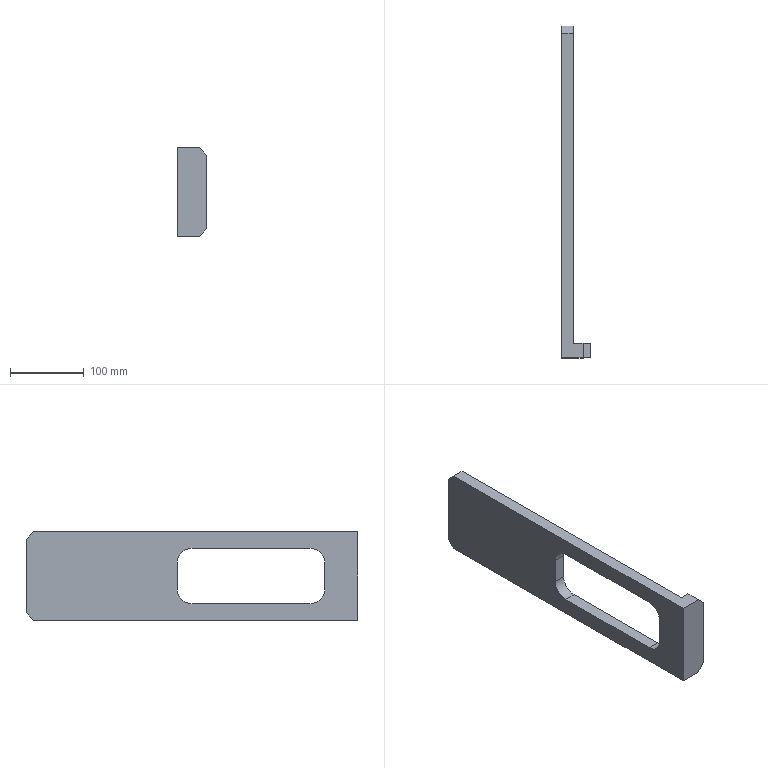Part | STEP file | PN_0019 | 1 solid | 20 faces | box 39.2 x 450 x 120 mm | volume 681574 mm3 | plane 16 | cylinder 4 | commonest cylinder face diameters 40 x4
STEP:
#1=CARTESIAN_POINT('',(0.,0.,0.));
#2=DIRECTION('',(0.,0.,1.));
#3=DIRECTION('',(1.,0.,0.));
#4=AXIS2_PLACEMENT_3D('',#1,#2,#3);
#5=CARTESIAN_POINT('',(0.,225.,97.5));
#6=VERTEX_POINT('',#5);
#7=CARTESIAN_POINT('',(0.,65.,97.5));
#8=VERTEX_POINT('',#7);
#9=CARTESIAN_POINT('',(0.,0.,97.5));
#10=DIRECTION('',(0.,-1.,0.));
#11=VECTOR('',#10,1.);
#12=LINE('',#9,#11);
#13=CARTESIAN_POINT('',(0.,0.,120.));
#14=DIRECTION('',(1.,0.,0.));
#15=DIRECTION('',(0.,0.,-1.));
#16=AXIS2_PLACEMENT_3D('',#13,#14,#15);
#17=PLANE('',#16);
#18=CARTESIAN_POINT('',(22.5,0.));
#19=DIRECTION('',(0.,-1.));
#20=VECTOR('',#19,1.);
#21=LINE('',#18,#20);
#22=(GEOMETRIC_REPRESENTATION_CONTEXT(2)PARAMETRIC_REPRESENTATION_CONTEXT()REPRESENTATION_CONTEXT('',''));
#23=DEFINITIONAL_REPRESENTATION('',(#21),#22);
#24=PCURVE('',#17,#23);
#25=CARTESIAN_POINT('',(-104.,245.,97.5));
#26=DIRECTION('',(0.,0.,1.));
#27=DIRECTION('',(0.,-1.,0.));
#28=AXIS2_PLACEMENT_3D('',#25,#26,#27);
#29=PLANE('',#28);
#30=CARTESIAN_POINT('',(245.,104.));
#31=DIRECTION('',(1.,0.));
#32=VECTOR('',#31,1.);
#33=LINE('',#30,#32);
#34=(GEOMETRIC_REPRESENTATION_CONTEXT(2)PARAMETRIC_REPRESENTATION_CONTEXT()REPRESENTATION_CONTEXT('',''));
#35=DEFINITIONAL_REPRESENTATION('',(#33),#34);
#36=PCURVE('',#29,#35);
#37=SURFACE_CURVE('',#12,(#24,#36),.PCURVE_S1.);
#38=EDGE_CURVE('',#6,#8,#37,.T.);
#39=ORIENTED_EDGE('',*,*,#38,.T.);
#40=CARTESIAN_POINT('',(0.,45.,77.5));
#41=VERTEX_POINT('',#40);
#42=CARTESIAN_POINT('',(0.,65.,77.5));
#43=DIRECTION('',(1.,0.,0.));
#44=DIRECTION('',(0.,0.,-1.));
#45=AXIS2_PLACEMENT_3D('',#42,#43,#44);
#46=CIRCLE('',#45,20.);
#47=CARTESIAN_POINT('',(42.5,65.));
#48=DIRECTION('',(1.,0.));
#49=AXIS2_PLACEMENT_2D('',#47,#48);
#50=CIRCLE('',#49,20.);
#51=(GEOMETRIC_REPRESENTATION_CONTEXT(2)PARAMETRIC_REPRESENTATION_CONTEXT()REPRESENTATION_CONTEXT('',''));
#52=DEFINITIONAL_REPRESENTATION('',(#50),#51);
#53=PCURVE('',#17,#52);
#54=CARTESIAN_POINT('',(-104.,65.,77.5));
#55=DIRECTION('',(-1.,0.,0.));
#56=DIRECTION('',(0.,-1.,0.));
#57=AXIS2_PLACEMENT_3D('',#54,#55,#56);
#58=CYLINDRICAL_SURFACE('',#57,20.);
#59=CARTESIAN_POINT('',(4.712,-104.));
#60=DIRECTION('',(-1.,0.));
#61=VECTOR('',#60,1.);
#62=LINE('',#59,#61);
#63=(GEOMETRIC_REPRESENTATION_CONTEXT(2)PARAMETRIC_REPRESENTATION_CONTEXT()REPRESENTATION_CONTEXT('',''));
#64=DEFINITIONAL_REPRESENTATION('',(#62),#63);
#65=PCURVE('',#58,#64);
#66=SURFACE_CURVE('',#46,(#53,#65),.PCURVE_S1.);
#67=EDGE_CURVE('',#8,#41,#66,.T.);
#68=ORIENTED_EDGE('',*,*,#67,.T.);
#69=CARTESIAN_POINT('',(0.,45.,42.5));
#70=VERTEX_POINT('',#69);
#71=CARTESIAN_POINT('',(0.,45.,120.));
#72=DIRECTION('',(0.,0.,-1.));
#73=VECTOR('',#72,1.);
#74=LINE('',#71,#73);
#75=CARTESIAN_POINT('',(0.,45.));
#76=DIRECTION('',(1.,0.));
#77=VECTOR('',#76,1.);
#78=LINE('',#75,#77);
#79=(GEOMETRIC_REPRESENTATION_CONTEXT(2)PARAMETRIC_REPRESENTATION_CONTEXT()REPRESENTATION_CONTEXT('',''));
#80=DEFINITIONAL_REPRESENTATION('',(#78),#79);
#81=PCURVE('',#17,#80);
#82=CARTESIAN_POINT('',(-104.,45.,97.5));
#83=DIRECTION('',(0.,-1.,0.));
#84=DIRECTION('',(0.,0.,-1.));
#85=AXIS2_PLACEMENT_3D('',#82,#83,#84);
#86=PLANE('',#85);
#87=CARTESIAN_POINT('',(-22.5,104.));
#88=DIRECTION('',(1.,0.));
#89=VECTOR('',#88,1.);
#90=LINE('',#87,#89);
#91=(GEOMETRIC_REPRESENTATION_CONTEXT(2)PARAMETRIC_REPRESENTATION_CONTEXT()REPRESENTATION_CONTEXT('',''));
#92=DEFINITIONAL_REPRESENTATION('',(#90),#91);
#93=PCURVE('',#86,#92);
#94=SURFACE_CURVE('',#74,(#81,#93),.PCURVE_S1.);
#95=EDGE_CURVE('',#41,#70,#94,.T.);
#96=ORIENTED_EDGE('',*,*,#95,.T.);
#97=CARTESIAN_POINT('',(0.,65.,22.5));
#98=VERTEX_POINT('',#97);
#99=CARTESIAN_POINT('',(0.,65.,42.5));
#100=DIRECTION('',(1.,0.,0.));
#101=DIRECTION('',(0.,0.,-1.));
#102=AXIS2_PLACEMENT_3D('',#99,#100,#101);
#103=CIRCLE('',#102,20.);
#104=CARTESIAN_POINT('',(77.5,65.));
#105=DIRECTION('',(1.,0.));
#106=AXIS2_PLACEMENT_2D('',#104,#105);
#107=CIRCLE('',#106,20.);
#108=(GEOMETRIC_REPRESENTATION_CONTEXT(2)PARAMETRIC_REPRESENTATION_CONTEXT()REPRESENTATION_CONTEXT('',''));
#109=DEFINITIONAL_REPRESENTATION('',(#107),#108);
#110=PCURVE('',#17,#109);
#111=CARTESIAN_POINT('',(-104.,65.,42.5));
#112=DIRECTION('',(-1.,0.,0.));
#113=DIRECTION('',(0.,-1.,0.));
#114=AXIS2_PLACEMENT_3D('',#111,#112,#113);
#115=CYLINDRICAL_SURFACE('',#114,20.);
#116=CARTESIAN_POINT('',(10.996,-104.));
#117=DIRECTION('',(-1.,0.));
#118=VECTOR('',#117,1.);
#119=LINE('',#116,#118);
#120=(GEOMETRIC_REPRESENTATION_CONTEXT(2)PARAMETRIC_REPRESENTATION_CONTEXT()REPRESENTATION_CONTEXT('',''));
#121=DEFINITIONAL_REPRESENTATION('',(#119),#120);
#122=PCURVE('',#115,#121);
#123=SURFACE_CURVE('',#103,(#110,#122),.PCURVE_S1.);
#124=EDGE_CURVE('',#70,#98,#123,.T.);
#125=ORIENTED_EDGE('',*,*,#124,.T.);
#126=CARTESIAN_POINT('',(0.,225.,22.5));
#127=VERTEX_POINT('',#126);
#128=CARTESIAN_POINT('',(0.,0.,22.5));
#129=DIRECTION('',(0.,1.,0.));
#130=VECTOR('',#129,1.);
#131=LINE('',#128,#130);
#132=CARTESIAN_POINT('',(97.5,0.));
#133=DIRECTION('',(0.,1.));
#134=VECTOR('',#133,1.);
#135=LINE('',#132,#134);
#136=(GEOMETRIC_REPRESENTATION_CONTEXT(2)PARAMETRIC_REPRESENTATION_CONTEXT()REPRESENTATION_CONTEXT('',''));
#137=DEFINITIONAL_REPRESENTATION('',(#135),#136);
#138=PCURVE('',#17,#137);
#139=CARTESIAN_POINT('',(-104.,245.,22.5));
#140=DIRECTION('',(0.,0.,-1.));
#141=DIRECTION('',(0.,1.,0.));
#142=AXIS2_PLACEMENT_3D('',#139,#140,#141);
#143=PLANE('',#142);
#144=CARTESIAN_POINT('',(-245.,104.));
#145=DIRECTION('',(1.,0.));
#146=VECTOR('',#145,1.);
#147=LINE('',#144,#146);
#148=(GEOMETRIC_REPRESENTATION_CONTEXT(2)PARAMETRIC_REPRESENTATION_CONTEXT()REPRESENTATION_CONTEXT('',''));
#149=DEFINITIONAL_REPRESENTATION('',(#147),#148);
#150=PCURVE('',#143,#149);
#151=SURFACE_CURVE('',#131,(#138,#150),.PCURVE_S1.);
#152=EDGE_CURVE('',#98,#127,#151,.T.);
#153=ORIENTED_EDGE('',*,*,#152,.T.);
#154=CARTESIAN_POINT('',(0.,245.,42.5));
#155=VERTEX_POINT('',#154);
#156=CARTESIAN_POINT('',(0.,225.,42.5));
#157=DIRECTION('',(1.,0.,0.));
#158=DIRECTION('',(0.,0.,-1.));
#159=AXIS2_PLACEMENT_3D('',#156,#157,#158);
#160=CIRCLE('',#159,20.);
#161=CARTESIAN_POINT('',(77.5,225.));
#162=DIRECTION('',(1.,0.));
#163=AXIS2_PLACEMENT_2D('',#161,#162);
#164=CIRCLE('',#163,20.);
#165=(GEOMETRIC_REPRESENTATION_CONTEXT(2)PARAMETRIC_REPRESENTATION_CONTEXT()REPRESENTATION_CONTEXT('',''));
#166=DEFINITIONAL_REPRESENTATION('',(#164),#165);
#167=PCURVE('',#17,#166);
#168=CARTESIAN_POINT('',(-104.,225.,42.5));
#169=DIRECTION('',(-1.,0.,0.));
#170=DIRECTION('',(0.,-1.,0.));
#171=AXIS2_PLACEMENT_3D('',#168,#169,#170);
#172=CYLINDRICAL_SURFACE('',#171,20.);
#173=CARTESIAN_POINT('',(4.712,-104.));
#174=DIRECTION('',(-1.,0.));
#175=VECTOR('',#174,1.);
#176=LINE('',#173,#175);
#177=(GEOMETRIC_REPRESENTATION_CONTEXT(2)PARAMETRIC_REPRESENTATION_CONTEXT()REPRESENTATION_CONTEXT('',''));
#178=DEFINITIONAL_REPRESENTATION('',(#176),#177);
#179=PCURVE('',#172,#178);
#180=SURFACE_CURVE('',#160,(#167,#179),.PCURVE_S1.);
#181=EDGE_CURVE('',#127,#155,#180,.T.);
#182=ORIENTED_EDGE('',*,*,#181,.T.);
#183=CARTESIAN_POINT('',(0.,245.,77.5));
#184=VERTEX_POINT('',#183);
#185=CARTESIAN_POINT('',(0.,245.,120.));
#186=DIRECTION('',(0.,0.,1.));
#187=VECTOR('',#186,1.);
#188=LINE('',#185,#187);
#189=CARTESIAN_POINT('',(0.,245.));
#190=DIRECTION('',(-1.,0.));
#191=VECTOR('',#190,1.);
#192=LINE('',#189,#191);
#193=(GEOMETRIC_REPRESENTATION_CONTEXT(2)PARAMETRIC_REPRESENTATION_CONTEXT()REPRESENTATION_CONTEXT('',''));
#194=DEFINITIONAL_REPRESENTATION('',(#192),#193);
#195=PCURVE('',#17,#194);
#196=CARTESIAN_POINT('',(-104.,245.,97.5));
#197=DIRECTION('',(0.,1.,0.));
#198=DIRECTION('',(-1.,0.,0.));
#199=AXIS2_PLACEMENT_3D('',#196,#197,#198);
#200=PLANE('',#199);
#201=CARTESIAN_POINT('',(-104.,22.5));
#202=DIRECTION('',(0.,1.));
#203=VECTOR('',#202,1.);
#204=LINE('',#201,#203);
#205=(GEOMETRIC_REPRESENTATION_CONTEXT(2)PARAMETRIC_REPRESENTATION_CONTEXT()REPRESENTATION_CONTEXT('',''));
#206=DEFINITIONAL_REPRESENTATION('',(#204),#205);
#207=PCURVE('',#200,#206);
#208=SURFACE_CURVE('',#188,(#195,#207),.PCURVE_S1.);
#209=EDGE_CURVE('',#155,#184,#208,.T.);
#210=ORIENTED_EDGE('',*,*,#209,.T.);
#211=CARTESIAN_POINT('',(0.,225.,77.5));
#212=DIRECTION('',(1.,0.,0.));
#213=DIRECTION('',(0.,0.,-1.));
#214=AXIS2_PLACEMENT_3D('',#211,#212,#213);
#215=CIRCLE('',#214,20.);
#216=CARTESIAN_POINT('',(42.5,225.));
#217=DIRECTION('',(1.,0.));
#218=AXIS2_PLACEMENT_2D('',#216,#217);
#219=CIRCLE('',#218,20.);
#220=(GEOMETRIC_REPRESENTATION_CONTEXT(2)PARAMETRIC_REPRESENTATION_CONTEXT()REPRESENTATION_CONTEXT('',''));
#221=DEFINITIONAL_REPRESENTATION('',(#219),#220);
#222=PCURVE('',#17,#221);
#223=CARTESIAN_POINT('',(-104.,225.,77.5));
#224=DIRECTION('',(-1.,0.,0.));
#225=DIRECTION('',(0.,-1.,0.));
#226=AXIS2_PLACEMENT_3D('',#223,#224,#225);
#227=CYLINDRICAL_SURFACE('',#226,20.);
#228=CARTESIAN_POINT('',(4.712,-104.));
#229=DIRECTION('',(-1.,0.));
#230=VECTOR('',#229,1.);
#231=LINE('',#228,#230);
#232=(GEOMETRIC_REPRESENTATION_CONTEXT(2)PARAMETRIC_REPRESENTATION_CONTEXT()REPRESENTATION_CONTEXT('',''));
#233=DEFINITIONAL_REPRESENTATION('',(#231),#232);
#234=PCURVE('',#227,#233);
#235=SURFACE_CURVE('',#215,(#222,#234),.PCURVE_S1.);
#236=EDGE_CURVE('',#184,#6,#235,.T.);
#237=ORIENTED_EDGE('',*,*,#236,.T.);
#238=EDGE_LOOP('',(#39,#68,#96,#125,#153,#182,#210,#237));
#239=FACE_BOUND('',#238,.T.);
#240=CARTESIAN_POINT('',(0.,450.,110.));
#241=VERTEX_POINT('',#240);
#242=CARTESIAN_POINT('',(0.,450.,10.));
#243=VERTEX_POINT('',#242);
#244=CARTESIAN_POINT('',(0.,450.,120.));
#245=DIRECTION('',(0.,0.,-1.));
#246=VECTOR('',#245,1.);
#247=LINE('',#244,#246);
#248=CARTESIAN_POINT('',(0.,450.));
#249=DIRECTION('',(1.,0.));
#250=VECTOR('',#249,1.);
#251=LINE('',#248,#250);
#252=(GEOMETRIC_REPRESENTATION_CONTEXT(2)PARAMETRIC_REPRESENTATION_CONTEXT()REPRESENTATION_CONTEXT('',''));
#253=DEFINITIONAL_REPRESENTATION('',(#251),#252);
#254=PCURVE('',#17,#253);
#255=CARTESIAN_POINT('',(0.,450.,120.));
#256=DIRECTION('',(0.,-1.,0.));
#257=DIRECTION('',(0.,0.,-1.));
#258=AXIS2_PLACEMENT_3D('',#255,#256,#257);
#259=PLANE('',#258);
#260=CARTESIAN_POINT('',(0.,0.));
#261=DIRECTION('',(1.,0.));
#262=VECTOR('',#261,1.);
#263=LINE('',#260,#262);
#264=(GEOMETRIC_REPRESENTATION_CONTEXT(2)PARAMETRIC_REPRESENTATION_CONTEXT()REPRESENTATION_CONTEXT('',''));
#265=DEFINITIONAL_REPRESENTATION('',(#263),#264);
#266=PCURVE('',#259,#265);
#267=SURFACE_CURVE('',#247,(#254,#266),.PCURVE_S1.);
#268=EDGE_CURVE('',#241,#243,#267,.T.);
#269=ORIENTED_EDGE('',*,*,#268,.T.);
#270=CARTESIAN_POINT('',(0.,440.,0.));
#271=VERTEX_POINT('',#270);
#272=CARTESIAN_POINT('',(0.,450.,10.));
#273=DIRECTION('',(0.,-0.7071,-0.7071));
#274=VECTOR('',#273,1.);
#275=LINE('',#272,#274);
#276=CARTESIAN_POINT('',(110.,450.));
#277=DIRECTION('',(0.7071,-0.7071));
#278=VECTOR('',#277,1.);
#279=LINE('',#276,#278);
#280=(GEOMETRIC_REPRESENTATION_CONTEXT(2)PARAMETRIC_REPRESENTATION_CONTEXT()REPRESENTATION_CONTEXT('',''));
#281=DEFINITIONAL_REPRESENTATION('',(#279),#280);
#282=PCURVE('',#17,#281);
#283=CARTESIAN_POINT('',(0.,450.,10.));
#284=DIRECTION('',(0.,0.7071,-0.7071));
#285=DIRECTION('',(0.,0.7071,0.7071));
#286=AXIS2_PLACEMENT_3D('',#283,#284,#285);
#287=PLANE('',#286);
#288=CARTESIAN_POINT('',(0.,0.));
#289=DIRECTION('',(-1.,0.));
#290=VECTOR('',#289,1.);
#291=LINE('',#288,#290);
#292=(GEOMETRIC_REPRESENTATION_CONTEXT(2)PARAMETRIC_REPRESENTATION_CONTEXT()REPRESENTATION_CONTEXT('',''));
#293=DEFINITIONAL_REPRESENTATION('',(#291),#292);
#294=PCURVE('',#287,#293);
#295=SURFACE_CURVE('',#275,(#282,#294),.PCURVE_S1.);
#296=EDGE_CURVE('',#243,#271,#295,.T.);
#297=ORIENTED_EDGE('',*,*,#296,.T.);
#298=CARTESIAN_POINT('',(0.,0.,0.));
#299=VERTEX_POINT('',#298);
#300=CARTESIAN_POINT('',(0.,0.,0.));
#301=DIRECTION('',(0.,-1.,0.));
#302=VECTOR('',#301,1.);
#303=LINE('',#300,#302);
#304=CARTESIAN_POINT('',(120.,0.));
#305=DIRECTION('',(0.,-1.));
#306=VECTOR('',#305,1.);
#307=LINE('',#304,#306);
#308=(GEOMETRIC_REPRESENTATION_CONTEXT(2)PARAMETRIC_REPRESENTATION_CONTEXT()REPRESENTATION_CONTEXT('',''));
#309=DEFINITIONAL_REPRESENTATION('',(#307),#308);
#310=PCURVE('',#17,#309);
#311=CARTESIAN_POINT('',(0.,450.,0.));
#312=DIRECTION('',(0.,0.,-1.));
#313=DIRECTION('',(-1.,0.,0.));
#314=AXIS2_PLACEMENT_3D('',#311,#312,#313);
#315=PLANE('',#314);
#316=CARTESIAN_POINT('',(0.,-450.));
#317=DIRECTION('',(0.,-1.));
#318=VECTOR('',#317,1.);
#319=LINE('',#316,#318);
#320=(GEOMETRIC_REPRESENTATION_CONTEXT(2)PARAMETRIC_REPRESENTATION_CONTEXT()REPRESENTATION_CONTEXT('',''));
#321=DEFINITIONAL_REPRESENTATION('',(#319),#320);
#322=PCURVE('',#315,#321);
#323=SURFACE_CURVE('',#303,(#310,#322),.PCURVE_S1.);
#324=EDGE_CURVE('',#271,#299,#323,.T.);
#325=ORIENTED_EDGE('',*,*,#324,.T.);
#326=CARTESIAN_POINT('',(0.,0.,120.));
#327=VERTEX_POINT('',#326);
#328=CARTESIAN_POINT('',(0.,0.,120.));
#329=DIRECTION('',(0.,0.,-1.));
#330=VECTOR('',#329,1.);
#331=LINE('',#328,#330);
#332=CARTESIAN_POINT('',(0.,0.));
#333=DIRECTION('',(1.,0.));
#334=VECTOR('',#333,1.);
#335=LINE('',#332,#334);
#336=(GEOMETRIC_REPRESENTATION_CONTEXT(2)PARAMETRIC_REPRESENTATION_CONTEXT()REPRESENTATION_CONTEXT('',''));
#337=DEFINITIONAL_REPRESENTATION('',(#335),#336);
#338=PCURVE('',#17,#337);
#339=CARTESIAN_POINT('',(0.,0.,120.));
#340=DIRECTION('',(0.,1.,0.));
#341=DIRECTION('',(0.,0.,1.));
#342=AXIS2_PLACEMENT_3D('',#339,#340,#341);
#343=PLANE('',#342);
#344=CARTESIAN_POINT('',(0.,0.));
#345=DIRECTION('',(-1.,0.));
#346=VECTOR('',#345,1.);
#347=LINE('',#344,#346);
#348=(GEOMETRIC_REPRESENTATION_CONTEXT(2)PARAMETRIC_REPRESENTATION_CONTEXT()REPRESENTATION_CONTEXT('',''));
#349=DEFINITIONAL_REPRESENTATION('',(#347),#348);
#350=PCURVE('',#343,#349);
#351=SURFACE_CURVE('',#331,(#338,#350),.PCURVE_S1.);
#352=EDGE_CURVE('',#327,#299,#351,.T.);
#353=ORIENTED_EDGE('',*,*,#352,.F.);
#354=CARTESIAN_POINT('',(0.,440.,120.));
#355=VERTEX_POINT('',#354);
#356=CARTESIAN_POINT('',(0.,0.,120.));
#357=DIRECTION('',(0.,-1.,0.));
#358=VECTOR('',#357,1.);
#359=LINE('',#356,#358);
#360=CARTESIAN_POINT('',(0.,0.));
#361=DIRECTION('',(0.,-1.));
#362=VECTOR('',#361,1.);
#363=LINE('',#360,#362);
#364=(GEOMETRIC_REPRESENTATION_CONTEXT(2)PARAMETRIC_REPRESENTATION_CONTEXT()REPRESENTATION_CONTEXT('',''));
#365=DEFINITIONAL_REPRESENTATION('',(#363),#364);
#366=PCURVE('',#17,#365);
#367=CARTESIAN_POINT('',(0.,450.,120.));
#368=DIRECTION('',(0.,0.,-1.));
#369=DIRECTION('',(-1.,0.,0.));
#370=AXIS2_PLACEMENT_3D('',#367,#368,#369);
#371=PLANE('',#370);
#372=CARTESIAN_POINT('',(0.,-450.));
#373=DIRECTION('',(0.,-1.));
#374=VECTOR('',#373,1.);
#375=LINE('',#372,#374);
#376=(GEOMETRIC_REPRESENTATION_CONTEXT(2)PARAMETRIC_REPRESENTATION_CONTEXT()REPRESENTATION_CONTEXT('',''));
#377=DEFINITIONAL_REPRESENTATION('',(#375),#376);
#378=PCURVE('',#371,#377);
#379=SURFACE_CURVE('',#359,(#366,#378),.PCURVE_S1.);
#380=EDGE_CURVE('',#355,#327,#379,.T.);
#381=ORIENTED_EDGE('',*,*,#380,.F.);
#382=CARTESIAN_POINT('',(0.,440.,120.));
#383=DIRECTION('',(0.,0.7071,-0.7071));
#384=VECTOR('',#383,1.);
#385=LINE('',#382,#384);
#386=CARTESIAN_POINT('',(0.,440.));
#387=DIRECTION('',(0.7071,0.7071));
#388=VECTOR('',#387,1.);
#389=LINE('',#386,#388);
#390=(GEOMETRIC_REPRESENTATION_CONTEXT(2)PARAMETRIC_REPRESENTATION_CONTEXT()REPRESENTATION_CONTEXT('',''));
#391=DEFINITIONAL_REPRESENTATION('',(#389),#390);
#392=PCURVE('',#17,#391);
#393=CARTESIAN_POINT('',(0.,440.,120.));
#394=DIRECTION('',(0.,-0.7071,-0.7071));
#395=DIRECTION('',(0.,0.7071,-0.7071));
#396=AXIS2_PLACEMENT_3D('',#393,#394,#395);
#397=PLANE('',#396);
#398=CARTESIAN_POINT('',(0.,0.));
#399=DIRECTION('',(1.,0.));
#400=VECTOR('',#399,1.);
#401=LINE('',#398,#400);
#402=(GEOMETRIC_REPRESENTATION_CONTEXT(2)PARAMETRIC_REPRESENTATION_CONTEXT()REPRESENTATION_CONTEXT('',''));
#403=DEFINITIONAL_REPRESENTATION('',(#401),#402);
#404=PCURVE('',#397,#403);
#405=SURFACE_CURVE('',#385,(#392,#404),.PCURVE_S1.);
#406=EDGE_CURVE('',#355,#241,#405,.T.);
#407=ORIENTED_EDGE('',*,*,#406,.T.);
#408=EDGE_LOOP('',(#269,#297,#325,#353,#381,#407));
#409=FACE_BOUND('',#408,.T.);
#410=ADVANCED_FACE('',(#239,#409),#17,.F.);
#411=CARTESIAN_POINT('',(29.2,0.,0.));
#412=VERTEX_POINT('',#411);
#413=CARTESIAN_POINT('',(0.,0.,0.));
#414=DIRECTION('',(1.,0.,0.));
#415=VECTOR('',#414,1.);
#416=LINE('',#413,#415);
#417=CARTESIAN_POINT('',(-120.,0.));
#418=DIRECTION('',(0.,1.));
#419=VECTOR('',#418,1.);
#420=LINE('',#417,#419);
#421=(GEOMETRIC_REPRESENTATION_CONTEXT(2)PARAMETRIC_REPRESENTATION_CONTEXT()REPRESENTATION_CONTEXT('',''));
#422=DEFINITIONAL_REPRESENTATION('',(#420),#421);
#423=PCURVE('',#343,#422);
#424=CARTESIAN_POINT('',(0.,-450.));
#425=DIRECTION('',(-1.,0.));
#426=VECTOR('',#425,1.);
#427=LINE('',#424,#426);
#428=(GEOMETRIC_REPRESENTATION_CONTEXT(2)PARAMETRIC_REPRESENTATION_CONTEXT()REPRESENTATION_CONTEXT('',''));
#429=DEFINITIONAL_REPRESENTATION('',(#427),#428);
#430=PCURVE('',#315,#429);
#431=SURFACE_CURVE('',#416,(#423,#430),.PCURVE_S1.);
#432=EDGE_CURVE('',#299,#412,#431,.T.);
#433=ORIENTED_EDGE('',*,*,#432,.T.);
#434=CARTESIAN_POINT('',(39.2,0.,10.));
#435=VERTEX_POINT('',#434);
#436=CARTESIAN_POINT('',(39.2,0.,10.));
#437=DIRECTION('',(0.7071,0.,0.7071));
#438=VECTOR('',#437,1.);
#439=LINE('',#436,#438);
#440=CARTESIAN_POINT('',(-110.,39.2));
#441=DIRECTION('',(0.7071,0.7071));
#442=VECTOR('',#441,1.);
#443=LINE('',#440,#442);
#444=(GEOMETRIC_REPRESENTATION_CONTEXT(2)PARAMETRIC_REPRESENTATION_CONTEXT()REPRESENTATION_CONTEXT('',''));
#445=DEFINITIONAL_REPRESENTATION('',(#443),#444);
#446=PCURVE('',#343,#445);
#447=CARTESIAN_POINT('',(39.2,0.,10.));
#448=DIRECTION('',(0.7071,0.,-0.7071));
#449=DIRECTION('',(-0.7071,0.,-0.7071));
#450=AXIS2_PLACEMENT_3D('',#447,#448,#449);
#451=PLANE('',#450);
#452=CARTESIAN_POINT('',(0.,0.));
#453=DIRECTION('',(-1.,0.));
#454=VECTOR('',#453,1.);
#455=LINE('',#452,#454);
#456=(GEOMETRIC_REPRESENTATION_CONTEXT(2)PARAMETRIC_REPRESENTATION_CONTEXT()REPRESENTATION_CONTEXT('',''));
#457=DEFINITIONAL_REPRESENTATION('',(#455),#456);
#458=PCURVE('',#451,#457);
#459=SURFACE_CURVE('',#439,(#446,#458),.PCURVE_S1.);
#460=EDGE_CURVE('',#412,#435,#459,.T.);
#461=ORIENTED_EDGE('',*,*,#460,.T.);
#462=CARTESIAN_POINT('',(39.2,0.,110.));
#463=VERTEX_POINT('',#462);
#464=CARTESIAN_POINT('',(39.2,0.,120.));
#465=DIRECTION('',(0.,0.,-1.));
#466=VECTOR('',#465,1.);
#467=LINE('',#464,#466);
#468=CARTESIAN_POINT('',(0.,39.2));
#469=DIRECTION('',(-1.,0.));
#470=VECTOR('',#469,1.);
#471=LINE('',#468,#470);
#472=(GEOMETRIC_REPRESENTATION_CONTEXT(2)PARAMETRIC_REPRESENTATION_CONTEXT()REPRESENTATION_CONTEXT('',''));
#473=DEFINITIONAL_REPRESENTATION('',(#471),#472);
#474=PCURVE('',#343,#473);
#475=CARTESIAN_POINT('',(39.2,0.,120.));
#476=DIRECTION('',(-1.,0.,0.));
#477=DIRECTION('',(0.,0.,1.));
#478=AXIS2_PLACEMENT_3D('',#475,#476,#477);
#479=PLANE('',#478);
#480=CARTESIAN_POINT('',(0.,0.));
#481=DIRECTION('',(-1.,0.));
#482=VECTOR('',#481,1.);
#483=LINE('',#480,#482);
#484=(GEOMETRIC_REPRESENTATION_CONTEXT(2)PARAMETRIC_REPRESENTATION_CONTEXT()REPRESENTATION_CONTEXT('',''));
#485=DEFINITIONAL_REPRESENTATION('',(#483),#484);
#486=PCURVE('',#479,#485);
#487=SURFACE_CURVE('',#467,(#474,#486),.PCURVE_S1.);
#488=EDGE_CURVE('',#463,#435,#487,.T.);
#489=ORIENTED_EDGE('',*,*,#488,.F.);
#490=CARTESIAN_POINT('',(29.2,0.,120.));
#491=VERTEX_POINT('',#490);
#492=CARTESIAN_POINT('',(29.2,0.,120.));
#493=DIRECTION('',(-0.7071,0.,0.7071));
#494=VECTOR('',#493,1.);
#495=LINE('',#492,#494);
#496=CARTESIAN_POINT('',(0.,29.2));
#497=DIRECTION('',(0.7071,-0.7071));
#498=VECTOR('',#497,1.);
#499=LINE('',#496,#498);
#500=(GEOMETRIC_REPRESENTATION_CONTEXT(2)PARAMETRIC_REPRESENTATION_CONTEXT()REPRESENTATION_CONTEXT('',''));
#501=DEFINITIONAL_REPRESENTATION('',(#499),#500);
#502=PCURVE('',#343,#501);
#503=CARTESIAN_POINT('',(29.2,450.,120.));
#504=DIRECTION('',(-0.7071,0.,-0.7071));
#505=DIRECTION('',(-0.7071,0.,0.7071));
#506=AXIS2_PLACEMENT_3D('',#503,#504,#505);
#507=PLANE('',#506);
#508=CARTESIAN_POINT('',(0.,-450.));
#509=DIRECTION('',(1.,0.));
#510=VECTOR('',#509,1.);
#511=LINE('',#508,#510);
#512=(GEOMETRIC_REPRESENTATION_CONTEXT(2)PARAMETRIC_REPRESENTATION_CONTEXT()REPRESENTATION_CONTEXT('',''));
#513=DEFINITIONAL_REPRESENTATION('',(#511),#512);
#514=PCURVE('',#507,#513);
#515=SURFACE_CURVE('',#495,(#502,#514),.PCURVE_S1.);
#516=EDGE_CURVE('',#463,#491,#515,.T.);
#517=ORIENTED_EDGE('',*,*,#516,.T.);
#518=CARTESIAN_POINT('',(0.,0.,120.));
#519=DIRECTION('',(1.,0.,0.));
#520=VECTOR('',#519,1.);
#521=LINE('',#518,#520);
#522=CARTESIAN_POINT('',(0.,0.));
#523=DIRECTION('',(0.,1.));
#524=VECTOR('',#523,1.);
#525=LINE('',#522,#524);
#526=(GEOMETRIC_REPRESENTATION_CONTEXT(2)PARAMETRIC_REPRESENTATION_CONTEXT()REPRESENTATION_CONTEXT('',''));
#527=DEFINITIONAL_REPRESENTATION('',(#525),#526);
#528=PCURVE('',#343,#527);
#529=CARTESIAN_POINT('',(0.,-450.));
#530=DIRECTION('',(-1.,0.));
#531=VECTOR('',#530,1.);
#532=LINE('',#529,#531);
#533=(GEOMETRIC_REPRESENTATION_CONTEXT(2)PARAMETRIC_REPRESENTATION_CONTEXT()REPRESENTATION_CONTEXT('',''));
#534=DEFINITIONAL_REPRESENTATION('',(#532),#533);
#535=PCURVE('',#371,#534);
#536=SURFACE_CURVE('',#521,(#528,#535),.PCURVE_S1.);
#537=EDGE_CURVE('',#327,#491,#536,.T.);
#538=ORIENTED_EDGE('',*,*,#537,.F.);
#539=ORIENTED_EDGE('',*,*,#352,.T.);
#540=EDGE_LOOP('',(#433,#461,#489,#517,#538,#539));
#541=FACE_BOUND('',#540,.T.);
#542=ADVANCED_FACE('',(#541),#343,.F.);
#543=ORIENTED_EDGE('',*,*,#488,.T.);
#544=CARTESIAN_POINT('',(39.2,20.,10.));
#545=VERTEX_POINT('',#544);
#546=CARTESIAN_POINT('',(39.2,20.,10.));
#547=DIRECTION('',(0.,1.,0.));
#548=VECTOR('',#547,1.);
#549=LINE('',#546,#548);
#550=CARTESIAN_POINT('',(-110.,20.));
#551=DIRECTION('',(0.,1.));
#552=VECTOR('',#551,1.);
#553=LINE('',#550,#552);
#554=(GEOMETRIC_REPRESENTATION_CONTEXT(2)PARAMETRIC_REPRESENTATION_CONTEXT()REPRESENTATION_CONTEXT('',''));
#555=DEFINITIONAL_REPRESENTATION('',(#553),#554);
#556=PCURVE('',#479,#555);
#557=CARTESIAN_POINT('',(0.,20.));
#558=DIRECTION('',(0.,1.));
#559=VECTOR('',#558,1.);
#560=LINE('',#557,#559);
#561=(GEOMETRIC_REPRESENTATION_CONTEXT(2)PARAMETRIC_REPRESENTATION_CONTEXT()REPRESENTATION_CONTEXT('',''));
#562=DEFINITIONAL_REPRESENTATION('',(#560),#561);
#563=PCURVE('',#451,#562);
#564=SURFACE_CURVE('',#549,(#556,#563),.PCURVE_S1.);
#565=EDGE_CURVE('',#435,#545,#564,.T.);
#566=ORIENTED_EDGE('',*,*,#565,.T.);
#567=CARTESIAN_POINT('',(39.2,20.,110.));
#568=VERTEX_POINT('',#567);
#569=CARTESIAN_POINT('',(39.2,20.,120.));
#570=DIRECTION('',(0.,0.,-1.));
#571=VECTOR('',#570,1.);
#572=LINE('',#569,#571);
#573=CARTESIAN_POINT('',(0.,20.));
#574=DIRECTION('',(-1.,0.));
#575=VECTOR('',#574,1.);
#576=LINE('',#573,#575);
#577=(GEOMETRIC_REPRESENTATION_CONTEXT(2)PARAMETRIC_REPRESENTATION_CONTEXT()REPRESENTATION_CONTEXT('',''));
#578=DEFINITIONAL_REPRESENTATION('',(#576),#577);
#579=PCURVE('',#479,#578);
#580=CARTESIAN_POINT('',(16.,20.,120.));
#581=DIRECTION('',(0.,-1.,0.));
#582=DIRECTION('',(0.,0.,-1.));
#583=AXIS2_PLACEMENT_3D('',#580,#581,#582);
#584=PLANE('',#583);
#585=CARTESIAN_POINT('',(0.,23.2));
#586=DIRECTION('',(1.,0.));
#587=VECTOR('',#586,1.);
#588=LINE('',#585,#587);
#589=(GEOMETRIC_REPRESENTATION_CONTEXT(2)PARAMETRIC_REPRESENTATION_CONTEXT()REPRESENTATION_CONTEXT('',''));
#590=DEFINITIONAL_REPRESENTATION('',(#588),#589);
#591=PCURVE('',#584,#590);
#592=SURFACE_CURVE('',#572,(#579,#591),.PCURVE_S1.);
#593=EDGE_CURVE('',#568,#545,#592,.T.);
#594=ORIENTED_EDGE('',*,*,#593,.F.);
#595=CARTESIAN_POINT('',(39.2,0.,110.));
#596=DIRECTION('',(0.,-1.,0.));
#597=VECTOR('',#596,1.);
#598=LINE('',#595,#597);
#599=CARTESIAN_POINT('',(-10.,0.));
#600=DIRECTION('',(0.,-1.));
#601=VECTOR('',#600,1.);
#602=LINE('',#599,#601);
#603=(GEOMETRIC_REPRESENTATION_CONTEXT(2)PARAMETRIC_REPRESENTATION_CONTEXT()REPRESENTATION_CONTEXT('',''));
#604=DEFINITIONAL_REPRESENTATION('',(#602),#603);
#605=PCURVE('',#479,#604);
#606=CARTESIAN_POINT('',(-14.142,-450.));
#607=DIRECTION('',(0.,-1.));
#608=VECTOR('',#607,1.);
#609=LINE('',#606,#608);
#610=(GEOMETRIC_REPRESENTATION_CONTEXT(2)PARAMETRIC_REPRESENTATION_CONTEXT()REPRESENTATION_CONTEXT('',''));
#611=DEFINITIONAL_REPRESENTATION('',(#609),#610);
#612=PCURVE('',#507,#611);
#613=SURFACE_CURVE('',#598,(#605,#612),.PCURVE_S1.);
#614=EDGE_CURVE('',#568,#463,#613,.T.);
#615=ORIENTED_EDGE('',*,*,#614,.T.);
#616=EDGE_LOOP('',(#543,#566,#594,#615));
#617=FACE_BOUND('',#616,.T.);
#618=ADVANCED_FACE('',(#617),#479,.F.);
#619=ORIENTED_EDGE('',*,*,#593,.T.);
#620=CARTESIAN_POINT('',(29.2,20.,0.));
#621=VERTEX_POINT('',#620);
#622=CARTESIAN_POINT('',(39.2,20.,10.));
#623=DIRECTION('',(-0.7071,0.,-0.7071));
#624=VECTOR('',#623,1.);
#625=LINE('',#622,#624);
#626=CARTESIAN_POINT('',(110.,23.2));
#627=DIRECTION('',(0.7071,-0.7071));
#628=VECTOR('',#627,1.);
#629=LINE('',#626,#628);
#630=(GEOMETRIC_REPRESENTATION_CONTEXT(2)PARAMETRIC_REPRESENTATION_CONTEXT()REPRESENTATION_CONTEXT('',''));
#631=DEFINITIONAL_REPRESENTATION('',(#629),#630);
#632=PCURVE('',#584,#631);
#633=CARTESIAN_POINT('',(0.,20.));
#634=DIRECTION('',(1.,0.));
#635=VECTOR('',#634,1.);
#636=LINE('',#633,#635);
#637=(GEOMETRIC_REPRESENTATION_CONTEXT(2)PARAMETRIC_REPRESENTATION_CONTEXT()REPRESENTATION_CONTEXT('',''));
#638=DEFINITIONAL_REPRESENTATION('',(#636),#637);
#639=PCURVE('',#451,#638);
#640=SURFACE_CURVE('',#625,(#632,#639),.PCURVE_S1.);
#641=EDGE_CURVE('',#545,#621,#640,.T.);
#642=ORIENTED_EDGE('',*,*,#641,.T.);
#643=CARTESIAN_POINT('',(16.,20.,0.));
#644=VERTEX_POINT('',#643);
#645=CARTESIAN_POINT('',(16.,20.,0.));
#646=DIRECTION('',(-1.,0.,0.));
#647=VECTOR('',#646,1.);
#648=LINE('',#645,#647);
#649=CARTESIAN_POINT('',(120.,0.));
#650=DIRECTION('',(0.,-1.));
#651=VECTOR('',#650,1.);
#652=LINE('',#649,#651);
#653=(GEOMETRIC_REPRESENTATION_CONTEXT(2)PARAMETRIC_REPRESENTATION_CONTEXT()REPRESENTATION_CONTEXT('',''));
#654=DEFINITIONAL_REPRESENTATION('',(#652),#653);
#655=PCURVE('',#584,#654);
#656=CARTESIAN_POINT('',(-16.,-430.));
#657=DIRECTION('',(1.,0.));
#658=VECTOR('',#657,1.);
#659=LINE('',#656,#658);
#660=(GEOMETRIC_REPRESENTATION_CONTEXT(2)PARAMETRIC_REPRESENTATION_CONTEXT()REPRESENTATION_CONTEXT('',''));
#661=DEFINITIONAL_REPRESENTATION('',(#659),#660);
#662=PCURVE('',#315,#661);
#663=SURFACE_CURVE('',#648,(#655,#662),.PCURVE_S1.);
#664=EDGE_CURVE('',#621,#644,#663,.T.);
#665=ORIENTED_EDGE('',*,*,#664,.T.);
#666=CARTESIAN_POINT('',(16.,20.,120.));
#667=VERTEX_POINT('',#666);
#668=CARTESIAN_POINT('',(16.,20.,120.));
#669=DIRECTION('',(0.,0.,-1.));
#670=VECTOR('',#669,1.);
#671=LINE('',#668,#670);
#672=CARTESIAN_POINT('',(0.,0.));
#673=DIRECTION('',(1.,0.));
#674=VECTOR('',#673,1.);
#675=LINE('',#672,#674);
#676=(GEOMETRIC_REPRESENTATION_CONTEXT(2)PARAMETRIC_REPRESENTATION_CONTEXT()REPRESENTATION_CONTEXT('',''));
#677=DEFINITIONAL_REPRESENTATION('',(#675),#676);
#678=PCURVE('',#584,#677);
#679=CARTESIAN_POINT('',(16.,450.,120.));
#680=DIRECTION('',(-1.,0.,0.));
#681=DIRECTION('',(0.,-1.,0.));
#682=AXIS2_PLACEMENT_3D('',#679,#680,#681);
#683=PLANE('',#682);
#684=CARTESIAN_POINT('',(430.,0.));
#685=DIRECTION('',(0.,-1.));
#686=VECTOR('',#685,1.);
#687=LINE('',#684,#686);
#688=(GEOMETRIC_REPRESENTATION_CONTEXT(2)PARAMETRIC_REPRESENTATION_CONTEXT()REPRESENTATION_CONTEXT('',''));
#689=DEFINITIONAL_REPRESENTATION('',(#687),#688);
#690=PCURVE('',#683,#689);
#691=SURFACE_CURVE('',#671,(#678,#690),.PCURVE_S1.);
#692=EDGE_CURVE('',#667,#644,#691,.T.);
#693=ORIENTED_EDGE('',*,*,#692,.F.);
#694=CARTESIAN_POINT('',(29.2,20.,120.));
#695=VERTEX_POINT('',#694);
#696=CARTESIAN_POINT('',(16.,20.,120.));
#697=DIRECTION('',(-1.,0.,0.));
#698=VECTOR('',#697,1.);
#699=LINE('',#696,#698);
#700=CARTESIAN_POINT('',(0.,0.));
#701=DIRECTION('',(0.,-1.));
#702=VECTOR('',#701,1.);
#703=LINE('',#700,#702);
#704=(GEOMETRIC_REPRESENTATION_CONTEXT(2)PARAMETRIC_REPRESENTATION_CONTEXT()REPRESENTATION_CONTEXT('',''));
#705=DEFINITIONAL_REPRESENTATION('',(#703),#704);
#706=PCURVE('',#584,#705);
#707=CARTESIAN_POINT('',(-16.,-430.));
#708=DIRECTION('',(1.,0.));
#709=VECTOR('',#708,1.);
#710=LINE('',#707,#709);
#711=(GEOMETRIC_REPRESENTATION_CONTEXT(2)PARAMETRIC_REPRESENTATION_CONTEXT()REPRESENTATION_CONTEXT('',''));
#712=DEFINITIONAL_REPRESENTATION('',(#710),#711);
#713=PCURVE('',#371,#712);
#714=SURFACE_CURVE('',#699,(#706,#713),.PCURVE_S1.);
#715=EDGE_CURVE('',#695,#667,#714,.T.);
#716=ORIENTED_EDGE('',*,*,#715,.F.);
#717=CARTESIAN_POINT('',(29.2,20.,120.));
#718=DIRECTION('',(0.7071,0.,-0.7071));
#719=VECTOR('',#718,1.);
#720=LINE('',#717,#719);
#721=CARTESIAN_POINT('',(0.,13.2));
#722=DIRECTION('',(0.7071,0.7071));
#723=VECTOR('',#722,1.);
#724=LINE('',#721,#723);
#725=(GEOMETRIC_REPRESENTATION_CONTEXT(2)PARAMETRIC_REPRESENTATION_CONTEXT()REPRESENTATION_CONTEXT('',''));
#726=DEFINITIONAL_REPRESENTATION('',(#724),#725);
#727=PCURVE('',#584,#726);
#728=CARTESIAN_POINT('',(0.,-430.));
#729=DIRECTION('',(-1.,0.));
#730=VECTOR('',#729,1.);
#731=LINE('',#728,#730);
#732=(GEOMETRIC_REPRESENTATION_CONTEXT(2)PARAMETRIC_REPRESENTATION_CONTEXT()REPRESENTATION_CONTEXT('',''));
#733=DEFINITIONAL_REPRESENTATION('',(#731),#732);
#734=PCURVE('',#507,#733);
#735=SURFACE_CURVE('',#720,(#727,#734),.PCURVE_S1.);
#736=EDGE_CURVE('',#695,#568,#735,.T.);
#737=ORIENTED_EDGE('',*,*,#736,.T.);
#738=EDGE_LOOP('',(#619,#642,#665,#693,#716,#737));
#739=FACE_BOUND('',#738,.T.);
#740=ADVANCED_FACE('',(#739),#584,.F.);
#741=CARTESIAN_POINT('',(16.,245.,42.5));
#742=VERTEX_POINT('',#741);
#743=CARTESIAN_POINT('',(16.,245.,77.5));
#744=VERTEX_POINT('',#743);
#745=CARTESIAN_POINT('',(16.,245.,97.5));
#746=DIRECTION('',(0.,0.,1.));
#747=VECTOR('',#746,1.);
#748=LINE('',#745,#747);
#749=CARTESIAN_POINT('',(205.,-22.5));
#750=DIRECTION('',(0.,1.));
#751=VECTOR('',#750,1.);
#752=LINE('',#749,#751);
#753=(GEOMETRIC_REPRESENTATION_CONTEXT(2)PARAMETRIC_REPRESENTATION_CONTEXT()REPRESENTATION_CONTEXT('',''));
#754=DEFINITIONAL_REPRESENTATION('',(#752),#753);
#755=PCURVE('',#683,#754);
#756=CARTESIAN_POINT('',(-120.,0.));
#757=DIRECTION('',(0.,1.));
#758=VECTOR('',#757,1.);
#759=LINE('',#756,#758);
#760=(GEOMETRIC_REPRESENTATION_CONTEXT(2)PARAMETRIC_REPRESENTATION_CONTEXT()REPRESENTATION_CONTEXT('',''));
#761=DEFINITIONAL_REPRESENTATION('',(#759),#760);
#762=PCURVE('',#200,#761);
#763=SURFACE_CURVE('',#748,(#755,#762),.PCURVE_S1.);
#764=EDGE_CURVE('',#742,#744,#763,.T.);
#765=ORIENTED_EDGE('',*,*,#764,.F.);
#766=CARTESIAN_POINT('',(16.,225.,22.5));
#767=VERTEX_POINT('',#766);
#768=CARTESIAN_POINT('',(16.,225.,42.5));
#769=DIRECTION('',(-1.,0.,0.));
#770=DIRECTION('',(0.,-1.,0.));
#771=AXIS2_PLACEMENT_3D('',#768,#769,#770);
#772=CIRCLE('',#771,20.);
#773=CARTESIAN_POINT('',(225.,-77.5));
#774=DIRECTION('',(1.,0.));
#775=AXIS2_PLACEMENT_2D('',#773,#774);
#776=CIRCLE('',#775,20.);
#777=(GEOMETRIC_REPRESENTATION_CONTEXT(2)PARAMETRIC_REPRESENTATION_CONTEXT()REPRESENTATION_CONTEXT('',''));
#778=DEFINITIONAL_REPRESENTATION('',(#776),#777);
#779=PCURVE('',#683,#778);
#780=CARTESIAN_POINT('',(0.,-120.));
#781=DIRECTION('',(1.,0.));
#782=VECTOR('',#781,1.);
#783=LINE('',#780,#782);
#784=(GEOMETRIC_REPRESENTATION_CONTEXT(2)PARAMETRIC_REPRESENTATION_CONTEXT()REPRESENTATION_CONTEXT('',''));
#785=DEFINITIONAL_REPRESENTATION('',(#783),#784);
#786=PCURVE('',#172,#785);
#787=SURFACE_CURVE('',#772,(#779,#786),.PCURVE_S1.);
#788=EDGE_CURVE('',#742,#767,#787,.T.);
#789=ORIENTED_EDGE('',*,*,#788,.T.);
#790=CARTESIAN_POINT('',(16.,65.,22.5));
#791=VERTEX_POINT('',#790);
#792=CARTESIAN_POINT('',(16.,245.,22.5));
#793=DIRECTION('',(0.,1.,0.));
#794=VECTOR('',#793,1.);
#795=LINE('',#792,#794);
#796=CARTESIAN_POINT('',(205.,-97.5));
#797=DIRECTION('',(-1.,0.));
#798=VECTOR('',#797,1.);
#799=LINE('',#796,#798);
#800=(GEOMETRIC_REPRESENTATION_CONTEXT(2)PARAMETRIC_REPRESENTATION_CONTEXT()REPRESENTATION_CONTEXT('',''));
#801=DEFINITIONAL_REPRESENTATION('',(#799),#800);
#802=PCURVE('',#683,#801);
#803=CARTESIAN_POINT('',(0.,120.));
#804=DIRECTION('',(1.,0.));
#805=VECTOR('',#804,1.);
#806=LINE('',#803,#805);
#807=(GEOMETRIC_REPRESENTATION_CONTEXT(2)PARAMETRIC_REPRESENTATION_CONTEXT()REPRESENTATION_CONTEXT('',''));
#808=DEFINITIONAL_REPRESENTATION('',(#806),#807);
#809=PCURVE('',#143,#808);
#810=SURFACE_CURVE('',#795,(#802,#809),.PCURVE_S1.);
#811=EDGE_CURVE('',#791,#767,#810,.T.);
#812=ORIENTED_EDGE('',*,*,#811,.F.);
#813=CARTESIAN_POINT('',(16.,45.,42.5));
#814=VERTEX_POINT('',#813);
#815=CARTESIAN_POINT('',(16.,65.,42.5));
#816=DIRECTION('',(-1.,0.,0.));
#817=DIRECTION('',(0.,-1.,0.));
#818=AXIS2_PLACEMENT_3D('',#815,#816,#817);
#819=CIRCLE('',#818,20.);
#820=CARTESIAN_POINT('',(385.,-77.5));
#821=DIRECTION('',(1.,0.));
#822=AXIS2_PLACEMENT_2D('',#820,#821);
#823=CIRCLE('',#822,20.);
#824=(GEOMETRIC_REPRESENTATION_CONTEXT(2)PARAMETRIC_REPRESENTATION_CONTEXT()REPRESENTATION_CONTEXT('',''));
#825=DEFINITIONAL_REPRESENTATION('',(#823),#824);
#826=PCURVE('',#683,#825);
#827=CARTESIAN_POINT('',(0.,-120.));
#828=DIRECTION('',(1.,0.));
#829=VECTOR('',#828,1.);
#830=LINE('',#827,#829);
#831=(GEOMETRIC_REPRESENTATION_CONTEXT(2)PARAMETRIC_REPRESENTATION_CONTEXT()REPRESENTATION_CONTEXT('',''));
#832=DEFINITIONAL_REPRESENTATION('',(#830),#831);
#833=PCURVE('',#115,#832);
#834=SURFACE_CURVE('',#819,(#826,#833),.PCURVE_S1.);
#835=EDGE_CURVE('',#791,#814,#834,.T.);
#836=ORIENTED_EDGE('',*,*,#835,.T.);
#837=CARTESIAN_POINT('',(16.,45.,77.5));
#838=VERTEX_POINT('',#837);
#839=CARTESIAN_POINT('',(16.,45.,97.5));
#840=DIRECTION('',(0.,0.,-1.));
#841=VECTOR('',#840,1.);
#842=LINE('',#839,#841);
#843=CARTESIAN_POINT('',(405.,-22.5));
#844=DIRECTION('',(0.,-1.));
#845=VECTOR('',#844,1.);
#846=LINE('',#843,#845);
#847=(GEOMETRIC_REPRESENTATION_CONTEXT(2)PARAMETRIC_REPRESENTATION_CONTEXT()REPRESENTATION_CONTEXT('',''));
#848=DEFINITIONAL_REPRESENTATION('',(#846),#847);
#849=PCURVE('',#683,#848);
#850=CARTESIAN_POINT('',(0.,120.));
#851=DIRECTION('',(1.,0.));
#852=VECTOR('',#851,1.);
#853=LINE('',#850,#852);
#854=(GEOMETRIC_REPRESENTATION_CONTEXT(2)PARAMETRIC_REPRESENTATION_CONTEXT()REPRESENTATION_CONTEXT('',''));
#855=DEFINITIONAL_REPRESENTATION('',(#853),#854);
#856=PCURVE('',#86,#855);
#857=SURFACE_CURVE('',#842,(#849,#856),.PCURVE_S1.);
#858=EDGE_CURVE('',#838,#814,#857,.T.);
#859=ORIENTED_EDGE('',*,*,#858,.F.);
#860=CARTESIAN_POINT('',(16.,65.,97.5));
#861=VERTEX_POINT('',#860);
#862=CARTESIAN_POINT('',(16.,65.,77.5));
#863=DIRECTION('',(-1.,0.,0.));
#864=DIRECTION('',(0.,-1.,0.));
#865=AXIS2_PLACEMENT_3D('',#862,#863,#864);
#866=CIRCLE('',#865,20.);
#867=CARTESIAN_POINT('',(385.,-42.5));
#868=DIRECTION('',(1.,0.));
#869=AXIS2_PLACEMENT_2D('',#867,#868);
#870=CIRCLE('',#869,20.);
#871=(GEOMETRIC_REPRESENTATION_CONTEXT(2)PARAMETRIC_REPRESENTATION_CONTEXT()REPRESENTATION_CONTEXT('',''));
#872=DEFINITIONAL_REPRESENTATION('',(#870),#871);
#873=PCURVE('',#683,#872);
#874=CARTESIAN_POINT('',(0.,-120.));
#875=DIRECTION('',(1.,0.));
#876=VECTOR('',#875,1.);
#877=LINE('',#874,#876);
#878=(GEOMETRIC_REPRESENTATION_CONTEXT(2)PARAMETRIC_REPRESENTATION_CONTEXT()REPRESENTATION_CONTEXT('',''));
#879=DEFINITIONAL_REPRESENTATION('',(#877),#878);
#880=PCURVE('',#58,#879);
#881=SURFACE_CURVE('',#866,(#873,#880),.PCURVE_S1.);
#882=EDGE_CURVE('',#838,#861,#881,.T.);
#883=ORIENTED_EDGE('',*,*,#882,.T.);
#884=CARTESIAN_POINT('',(16.,225.,97.5));
#885=VERTEX_POINT('',#884);
#886=CARTESIAN_POINT('',(16.,245.,97.5));
#887=DIRECTION('',(0.,-1.,0.));
#888=VECTOR('',#887,1.);
#889=LINE('',#886,#888);
#890=CARTESIAN_POINT('',(205.,-22.5));
#891=DIRECTION('',(1.,0.));
#892=VECTOR('',#891,1.);
#893=LINE('',#890,#892);
#894=(GEOMETRIC_REPRESENTATION_CONTEXT(2)PARAMETRIC_REPRESENTATION_CONTEXT()REPRESENTATION_CONTEXT('',''));
#895=DEFINITIONAL_REPRESENTATION('',(#893),#894);
#896=PCURVE('',#683,#895);
#897=CARTESIAN_POINT('',(0.,120.));
#898=DIRECTION('',(1.,0.));
#899=VECTOR('',#898,1.);
#900=LINE('',#897,#899);
#901=(GEOMETRIC_REPRESENTATION_CONTEXT(2)PARAMETRIC_REPRESENTATION_CONTEXT()REPRESENTATION_CONTEXT('',''));
#902=DEFINITIONAL_REPRESENTATION('',(#900),#901);
#903=PCURVE('',#29,#902);
#904=SURFACE_CURVE('',#889,(#896,#903),.PCURVE_S1.);
#905=EDGE_CURVE('',#885,#861,#904,.T.);
#906=ORIENTED_EDGE('',*,*,#905,.F.);
#907=CARTESIAN_POINT('',(16.,225.,77.5));
#908=DIRECTION('',(-1.,0.,0.));
#909=DIRECTION('',(0.,-1.,0.));
#910=AXIS2_PLACEMENT_3D('',#907,#908,#909);
#911=CIRCLE('',#910,20.);
#912=CARTESIAN_POINT('',(225.,-42.5));
#913=DIRECTION('',(1.,0.));
#914=AXIS2_PLACEMENT_2D('',#912,#913);
#915=CIRCLE('',#914,20.);
#916=(GEOMETRIC_REPRESENTATION_CONTEXT(2)PARAMETRIC_REPRESENTATION_CONTEXT()REPRESENTATION_CONTEXT('',''));
#917=DEFINITIONAL_REPRESENTATION('',(#915),#916);
#918=PCURVE('',#683,#917);
#919=CARTESIAN_POINT('',(0.,-120.));
#920=DIRECTION('',(1.,0.));
#921=VECTOR('',#920,1.);
#922=LINE('',#919,#921);
#923=(GEOMETRIC_REPRESENTATION_CONTEXT(2)PARAMETRIC_REPRESENTATION_CONTEXT()REPRESENTATION_CONTEXT('',''));
#924=DEFINITIONAL_REPRESENTATION('',(#922),#923);
#925=PCURVE('',#227,#924);
#926=SURFACE_CURVE('',#911,(#918,#925),.PCURVE_S1.);
#927=EDGE_CURVE('',#885,#744,#926,.T.);
#928=ORIENTED_EDGE('',*,*,#927,.T.);
#929=EDGE_LOOP('',(#765,#789,#812,#836,#859,#883,#906,#928));
#930=FACE_BOUND('',#929,.T.);
#931=CARTESIAN_POINT('',(16.,440.,0.));
#932=VERTEX_POINT('',#931);
#933=CARTESIAN_POINT('',(16.,450.,0.));
#934=DIRECTION('',(0.,1.,0.));
#935=VECTOR('',#934,1.);
#936=LINE('',#933,#935);
#937=CARTESIAN_POINT('',(0.,-120.));
#938=DIRECTION('',(-1.,0.));
#939=VECTOR('',#938,1.);
#940=LINE('',#937,#939);
#941=(GEOMETRIC_REPRESENTATION_CONTEXT(2)PARAMETRIC_REPRESENTATION_CONTEXT()REPRESENTATION_CONTEXT('',''));
#942=DEFINITIONAL_REPRESENTATION('',(#940),#941);
#943=PCURVE('',#683,#942);
#944=CARTESIAN_POINT('',(-16.,0.));
#945=DIRECTION('',(0.,1.));
#946=VECTOR('',#945,1.);
#947=LINE('',#944,#946);
#948=(GEOMETRIC_REPRESENTATION_CONTEXT(2)PARAMETRIC_REPRESENTATION_CONTEXT()REPRESENTATION_CONTEXT('',''));
#949=DEFINITIONAL_REPRESENTATION('',(#947),#948);
#950=PCURVE('',#315,#949);
#951=SURFACE_CURVE('',#936,(#943,#950),.PCURVE_S1.);
#952=EDGE_CURVE('',#644,#932,#951,.T.);
#953=ORIENTED_EDGE('',*,*,#952,.T.);
#954=CARTESIAN_POINT('',(16.,450.,10.));
#955=VERTEX_POINT('',#954);
#956=CARTESIAN_POINT('',(16.,450.,10.));
#957=DIRECTION('',(0.,0.7071,0.7071));
#958=VECTOR('',#957,1.);
#959=LINE('',#956,#958);
#960=CARTESIAN_POINT('',(0.,-110.));
#961=DIRECTION('',(-0.7071,0.7071));
#962=VECTOR('',#961,1.);
#963=LINE('',#960,#962);
#964=(GEOMETRIC_REPRESENTATION_CONTEXT(2)PARAMETRIC_REPRESENTATION_CONTEXT()REPRESENTATION_CONTEXT('',''));
#965=DEFINITIONAL_REPRESENTATION('',(#963),#964);
#966=PCURVE('',#683,#965);
#967=CARTESIAN_POINT('',(0.,16.));
#968=DIRECTION('',(1.,0.));
#969=VECTOR('',#968,1.);
#970=LINE('',#967,#969);
#971=(GEOMETRIC_REPRESENTATION_CONTEXT(2)PARAMETRIC_REPRESENTATION_CONTEXT()REPRESENTATION_CONTEXT('',''));
#972=DEFINITIONAL_REPRESENTATION('',(#970),#971);
#973=PCURVE('',#287,#972);
#974=SURFACE_CURVE('',#959,(#966,#973),.PCURVE_S1.);
#975=EDGE_CURVE('',#932,#955,#974,.T.);
#976=ORIENTED_EDGE('',*,*,#975,.T.);
#977=CARTESIAN_POINT('',(16.,450.,110.));
#978=VERTEX_POINT('',#977);
#979=CARTESIAN_POINT('',(16.,450.,120.));
#980=DIRECTION('',(0.,0.,-1.));
#981=VECTOR('',#980,1.);
#982=LINE('',#979,#981);
#983=CARTESIAN_POINT('',(0.,0.));
#984=DIRECTION('',(0.,-1.));
#985=VECTOR('',#984,1.);
#986=LINE('',#983,#985);
#987=(GEOMETRIC_REPRESENTATION_CONTEXT(2)PARAMETRIC_REPRESENTATION_CONTEXT()REPRESENTATION_CONTEXT('',''));
#988=DEFINITIONAL_REPRESENTATION('',(#986),#987);
#989=PCURVE('',#683,#988);
#990=CARTESIAN_POINT('',(0.,16.));
#991=DIRECTION('',(1.,0.));
#992=VECTOR('',#991,1.);
#993=LINE('',#990,#992);
#994=(GEOMETRIC_REPRESENTATION_CONTEXT(2)PARAMETRIC_REPRESENTATION_CONTEXT()REPRESENTATION_CONTEXT('',''));
#995=DEFINITIONAL_REPRESENTATION('',(#993),#994);
#996=PCURVE('',#259,#995);
#997=SURFACE_CURVE('',#982,(#989,#996),.PCURVE_S1.);
#998=EDGE_CURVE('',#978,#955,#997,.T.);
#999=ORIENTED_EDGE('',*,*,#998,.F.);
#1000=CARTESIAN_POINT('',(16.,440.,120.));
#1001=VERTEX_POINT('',#1000);
#1002=CARTESIAN_POINT('',(16.,440.,120.));
#1003=DIRECTION('',(0.,-0.7071,0.7071));
#1004=VECTOR('',#1003,1.);
#1005=LINE('',#1002,#1004);
#1006=CARTESIAN_POINT('',(10.,0.));
#1007=DIRECTION('',(0.7071,0.7071));
#1008=VECTOR('',#1007,1.);
#1009=LINE('',#1006,#1008);
#1010=(GEOMETRIC_REPRESENTATION_CONTEXT(2)PARAMETRIC_REPRESENTATION_CONTEXT()REPRESENTATION_CONTEXT('',''));
#1011=DEFINITIONAL_REPRESENTATION('',(#1009),#1010);
#1012=PCURVE('',#683,#1011);
#1013=CARTESIAN_POINT('',(0.,16.));
#1014=DIRECTION('',(-1.,0.));
#1015=VECTOR('',#1014,1.);
#1016=LINE('',#1013,#1015);
#1017=(GEOMETRIC_REPRESENTATION_CONTEXT(2)PARAMETRIC_REPRESENTATION_CONTEXT()REPRESENTATION_CONTEXT('',''));
#1018=DEFINITIONAL_REPRESENTATION('',(#1016),#1017);
#1019=PCURVE('',#397,#1018);
#1020=SURFACE_CURVE('',#1005,(#1012,#1019),.PCURVE_S1.);
#1021=EDGE_CURVE('',#978,#1001,#1020,.T.);
#1022=ORIENTED_EDGE('',*,*,#1021,.T.);
#1023=CARTESIAN_POINT('',(16.,450.,120.));
#1024=DIRECTION('',(0.,1.,0.));
#1025=VECTOR('',#1024,1.);
#1026=LINE('',#1023,#1025);
#1027=CARTESIAN_POINT('',(0.,0.));
#1028=DIRECTION('',(-1.,0.));
#1029=VECTOR('',#1028,1.);
#1030=LINE('',#1027,#1029);
#1031=(GEOMETRIC_REPRESENTATION_CONTEXT(2)PARAMETRIC_REPRESENTATION_CONTEXT()REPRESENTATION_CONTEXT('',''));
#1032=DEFINITIONAL_REPRESENTATION('',(#1030),#1031);
#1033=PCURVE('',#683,#1032);
#1034=CARTESIAN_POINT('',(-16.,0.));
#1035=DIRECTION('',(0.,1.));
#1036=VECTOR('',#1035,1.);
#1037=LINE('',#1034,#1036);
#1038=(GEOMETRIC_REPRESENTATION_CONTEXT(2)PARAMETRIC_REPRESENTATION_CONTEXT()REPRESENTATION_CONTEXT('',''));
#1039=DEFINITIONAL_REPRESENTATION('',(#1037),#1038);
#1040=PCURVE('',#371,#1039);
#1041=SURFACE_CURVE('',#1026,(#1033,#1040),.PCURVE_S1.);
#1042=EDGE_CURVE('',#667,#1001,#1041,.T.);
#1043=ORIENTED_EDGE('',*,*,#1042,.F.);
#1044=ORIENTED_EDGE('',*,*,#692,.T.);
#1045=EDGE_LOOP('',(#953,#976,#999,#1022,#1043,#1044));
#1046=FACE_BOUND('',#1045,.T.);
#1047=ADVANCED_FACE('',(#930,#1046),#683,.F.);
#1048=ORIENTED_EDGE('',*,*,#998,.T.);
#1049=CARTESIAN_POINT('',(0.,450.,10.));
#1050=DIRECTION('',(-1.,0.,0.));
#1051=VECTOR('',#1050,1.);
#1052=LINE('',#1049,#1051);
#1053=CARTESIAN_POINT('',(110.,0.));
#1054=DIRECTION('',(0.,-1.));
#1055=VECTOR('',#1054,1.);
#1056=LINE('',#1053,#1055);
#1057=(GEOMETRIC_REPRESENTATION_CONTEXT(2)PARAMETRIC_REPRESENTATION_CONTEXT()REPRESENTATION_CONTEXT('',''));
#1058=DEFINITIONAL_REPRESENTATION('',(#1056),#1057);
#1059=PCURVE('',#259,#1058);
#1060=CARTESIAN_POINT('',(0.,0.));
#1061=DIRECTION('',(0.,-1.));
#1062=VECTOR('',#1061,1.);
#1063=LINE('',#1060,#1062);
#1064=(GEOMETRIC_REPRESENTATION_CONTEXT(2)PARAMETRIC_REPRESENTATION_CONTEXT()REPRESENTATION_CONTEXT('',''));
#1065=DEFINITIONAL_REPRESENTATION('',(#1063),#1064);
#1066=PCURVE('',#287,#1065);
#1067=SURFACE_CURVE('',#1052,(#1059,#1066),.PCURVE_S1.);
#1068=EDGE_CURVE('',#955,#243,#1067,.T.);
#1069=ORIENTED_EDGE('',*,*,#1068,.T.);
#1070=ORIENTED_EDGE('',*,*,#268,.F.);
#1071=CARTESIAN_POINT('',(0.,450.,110.));
#1072=DIRECTION('',(1.,0.,0.));
#1073=VECTOR('',#1072,1.);
#1074=LINE('',#1071,#1073);
#1075=CARTESIAN_POINT('',(10.,0.));
#1076=DIRECTION('',(0.,1.));
#1077=VECTOR('',#1076,1.);
#1078=LINE('',#1075,#1077);
#1079=(GEOMETRIC_REPRESENTATION_CONTEXT(2)PARAMETRIC_REPRESENTATION_CONTEXT()REPRESENTATION_CONTEXT('',''));
#1080=DEFINITIONAL_REPRESENTATION('',(#1078),#1079);
#1081=PCURVE('',#259,#1080);
#1082=CARTESIAN_POINT('',(14.142,0.));
#1083=DIRECTION('',(0.,1.));
#1084=VECTOR('',#1083,1.);
#1085=LINE('',#1082,#1084);
#1086=(GEOMETRIC_REPRESENTATION_CONTEXT(2)PARAMETRIC_REPRESENTATION_CONTEXT()REPRESENTATION_CONTEXT('',''));
#1087=DEFINITIONAL_REPRESENTATION('',(#1085),#1086);
#1088=PCURVE('',#397,#1087);
#1089=SURFACE_CURVE('',#1074,(#1081,#1088),.PCURVE_S1.);
#1090=EDGE_CURVE('',#241,#978,#1089,.T.);
#1091=ORIENTED_EDGE('',*,*,#1090,.T.);
#1092=EDGE_LOOP('',(#1048,#1069,#1070,#1091));
#1093=FACE_BOUND('',#1092,.T.);
#1094=ADVANCED_FACE('',(#1093),#259,.F.);
#1095=ORIENTED_EDGE('',*,*,#537,.T.);
#1096=CARTESIAN_POINT('',(29.2,450.,120.));
#1097=DIRECTION('',(0.,1.,0.));
#1098=VECTOR('',#1097,1.);
#1099=LINE('',#1096,#1098);
#1100=CARTESIAN_POINT('',(-29.2,0.));
#1101=DIRECTION('',(0.,1.));
#1102=VECTOR('',#1101,1.);
#1103=LINE('',#1100,#1102);
#1104=(GEOMETRIC_REPRESENTATION_CONTEXT(2)PARAMETRIC_REPRESENTATION_CONTEXT()REPRESENTATION_CONTEXT('',''));
#1105=DEFINITIONAL_REPRESENTATION('',(#1103),#1104);
#1106=PCURVE('',#371,#1105);
#1107=CARTESIAN_POINT('',(0.,0.));
#1108=DIRECTION('',(0.,1.));
#1109=VECTOR('',#1108,1.);
#1110=LINE('',#1107,#1109);
#1111=(GEOMETRIC_REPRESENTATION_CONTEXT(2)PARAMETRIC_REPRESENTATION_CONTEXT()REPRESENTATION_CONTEXT('',''));
#1112=DEFINITIONAL_REPRESENTATION('',(#1110),#1111);
#1113=PCURVE('',#507,#1112);
#1114=SURFACE_CURVE('',#1099,(#1106,#1113),.PCURVE_S1.);
#1115=EDGE_CURVE('',#491,#695,#1114,.T.);
#1116=ORIENTED_EDGE('',*,*,#1115,.T.);
#1117=ORIENTED_EDGE('',*,*,#715,.T.);
#1118=ORIENTED_EDGE('',*,*,#1042,.T.);
#1119=CARTESIAN_POINT('',(0.,440.,120.));
#1120=DIRECTION('',(-1.,0.,0.));
#1121=VECTOR('',#1120,1.);
#1122=LINE('',#1119,#1121);
#1123=CARTESIAN_POINT('',(0.,-10.));
#1124=DIRECTION('',(1.,0.));
#1125=VECTOR('',#1124,1.);
#1126=LINE('',#1123,#1125);
#1127=(GEOMETRIC_REPRESENTATION_CONTEXT(2)PARAMETRIC_REPRESENTATION_CONTEXT()REPRESENTATION_CONTEXT('',''));
#1128=DEFINITIONAL_REPRESENTATION('',(#1126),#1127);
#1129=PCURVE('',#371,#1128);
#1130=CARTESIAN_POINT('',(0.,0.));
#1131=DIRECTION('',(0.,-1.));
#1132=VECTOR('',#1131,1.);
#1133=LINE('',#1130,#1132);
#1134=(GEOMETRIC_REPRESENTATION_CONTEXT(2)PARAMETRIC_REPRESENTATION_CONTEXT()REPRESENTATION_CONTEXT('',''));
#1135=DEFINITIONAL_REPRESENTATION('',(#1133),#1134);
#1136=PCURVE('',#397,#1135);
#1137=SURFACE_CURVE('',#1122,(#1129,#1136),.PCURVE_S1.);
#1138=EDGE_CURVE('',#1001,#355,#1137,.T.);
#1139=ORIENTED_EDGE('',*,*,#1138,.T.);
#1140=ORIENTED_EDGE('',*,*,#380,.T.);
#1141=EDGE_LOOP('',(#1095,#1116,#1117,#1118,#1139,#1140));
#1142=FACE_BOUND('',#1141,.T.);
#1143=ADVANCED_FACE('',(#1142),#371,.F.);
#1144=ORIENTED_EDGE('',*,*,#664,.F.);
#1145=CARTESIAN_POINT('',(29.2,0.,0.));
#1146=DIRECTION('',(0.,-1.,0.));
#1147=VECTOR('',#1146,1.);
#1148=LINE('',#1145,#1147);
#1149=CARTESIAN_POINT('',(-29.2,-450.));
#1150=DIRECTION('',(0.,-1.));
#1151=VECTOR('',#1150,1.);
#1152=LINE('',#1149,#1151);
#1153=(GEOMETRIC_REPRESENTATION_CONTEXT(2)PARAMETRIC_REPRESENTATION_CONTEXT()REPRESENTATION_CONTEXT('',''));
#1154=DEFINITIONAL_REPRESENTATION('',(#1152),#1153);
#1155=PCURVE('',#315,#1154);
#1156=CARTESIAN_POINT('',(14.142,0.));
#1157=DIRECTION('',(0.,-1.));
#1158=VECTOR('',#1157,1.);
#1159=LINE('',#1156,#1158);
#1160=(GEOMETRIC_REPRESENTATION_CONTEXT(2)PARAMETRIC_REPRESENTATION_CONTEXT()REPRESENTATION_CONTEXT('',''));
#1161=DEFINITIONAL_REPRESENTATION('',(#1159),#1160);
#1162=PCURVE('',#451,#1161);
#1163=SURFACE_CURVE('',#1148,(#1155,#1162),.PCURVE_S1.);
#1164=EDGE_CURVE('',#621,#412,#1163,.T.);
#1165=ORIENTED_EDGE('',*,*,#1164,.T.);
#1166=ORIENTED_EDGE('',*,*,#432,.F.);
#1167=ORIENTED_EDGE('',*,*,#324,.F.);
#1168=CARTESIAN_POINT('',(16.,440.,0.));
#1169=DIRECTION('',(1.,0.,0.));
#1170=VECTOR('',#1169,1.);
#1171=LINE('',#1168,#1170);
#1172=CARTESIAN_POINT('',(-16.,-10.));
#1173=DIRECTION('',(-1.,0.));
#1174=VECTOR('',#1173,1.);
#1175=LINE('',#1172,#1174);
#1176=(GEOMETRIC_REPRESENTATION_CONTEXT(2)PARAMETRIC_REPRESENTATION_CONTEXT()REPRESENTATION_CONTEXT('',''));
#1177=DEFINITIONAL_REPRESENTATION('',(#1175),#1176);
#1178=PCURVE('',#315,#1177);
#1179=CARTESIAN_POINT('',(-14.142,16.));
#1180=DIRECTION('',(0.,1.));
#1181=VECTOR('',#1180,1.);
#1182=LINE('',#1179,#1181);
#1183=(GEOMETRIC_REPRESENTATION_CONTEXT(2)PARAMETRIC_REPRESENTATION_CONTEXT()REPRESENTATION_CONTEXT('',''));
#1184=DEFINITIONAL_REPRESENTATION('',(#1182),#1183);
#1185=PCURVE('',#287,#1184);
#1186=SURFACE_CURVE('',#1171,(#1178,#1185),.PCURVE_S1.);
#1187=EDGE_CURVE('',#271,#932,#1186,.T.);
#1188=ORIENTED_EDGE('',*,*,#1187,.T.);
#1189=ORIENTED_EDGE('',*,*,#952,.F.);
#1190=EDGE_LOOP('',(#1144,#1165,#1166,#1167,#1188,#1189));
#1191=FACE_BOUND('',#1190,.T.);
#1192=ADVANCED_FACE('',(#1191),#315,.T.);
#1193=ORIENTED_EDGE('',*,*,#460,.F.);
#1194=ORIENTED_EDGE('',*,*,#1164,.F.);
#1195=ORIENTED_EDGE('',*,*,#641,.F.);
#1196=ORIENTED_EDGE('',*,*,#565,.F.);
#1197=EDGE_LOOP('',(#1193,#1194,#1195,#1196));
#1198=FACE_BOUND('',#1197,.T.);
#1199=ADVANCED_FACE('',(#1198),#451,.T.);
#1200=ORIENTED_EDGE('',*,*,#516,.F.);
#1201=ORIENTED_EDGE('',*,*,#614,.F.);
#1202=ORIENTED_EDGE('',*,*,#736,.F.);
#1203=ORIENTED_EDGE('',*,*,#1115,.F.);
#1204=EDGE_LOOP('',(#1200,#1201,#1202,#1203));
#1205=FACE_BOUND('',#1204,.T.);
#1206=ADVANCED_FACE('',(#1205),#507,.F.);
#1207=ORIENTED_EDGE('',*,*,#975,.F.);
#1208=ORIENTED_EDGE('',*,*,#1187,.F.);
#1209=ORIENTED_EDGE('',*,*,#296,.F.);
#1210=ORIENTED_EDGE('',*,*,#1068,.F.);
#1211=EDGE_LOOP('',(#1207,#1208,#1209,#1210));
#1212=FACE_BOUND('',#1211,.T.);
#1213=ADVANCED_FACE('',(#1212),#287,.T.);
#1214=ORIENTED_EDGE('',*,*,#1021,.F.);
#1215=ORIENTED_EDGE('',*,*,#1090,.F.);
#1216=ORIENTED_EDGE('',*,*,#406,.F.);
#1217=ORIENTED_EDGE('',*,*,#1138,.F.);
#1218=EDGE_LOOP('',(#1214,#1215,#1216,#1217));
#1219=FACE_BOUND('',#1218,.T.);
#1220=ADVANCED_FACE('',(#1219),#397,.F.);
#1221=ORIENTED_EDGE('',*,*,#811,.T.);
#1222=CARTESIAN_POINT('',(0.,225.,22.5));
#1223=DIRECTION('',(-1.,0.,0.));
#1224=VECTOR('',#1223,1.);
#1225=LINE('',#1222,#1224);
#1226=CARTESIAN_POINT('',(-20.,104.));
#1227=DIRECTION('',(0.,-1.));
#1228=VECTOR('',#1227,1.);
#1229=LINE('',#1226,#1228);
#1230=(GEOMETRIC_REPRESENTATION_CONTEXT(2)PARAMETRIC_REPRESENTATION_CONTEXT()REPRESENTATION_CONTEXT('',''));
#1231=DEFINITIONAL_REPRESENTATION('',(#1229),#1230);
#1232=PCURVE('',#143,#1231);
#1233=CARTESIAN_POINT('',(4.712,-104.));
#1234=DIRECTION('',(0.,1.));
#1235=VECTOR('',#1234,1.);
#1236=LINE('',#1233,#1235);
#1237=(GEOMETRIC_REPRESENTATION_CONTEXT(2)PARAMETRIC_REPRESENTATION_CONTEXT()REPRESENTATION_CONTEXT('',''));
#1238=DEFINITIONAL_REPRESENTATION('',(#1236),#1237);
#1239=PCURVE('',#172,#1238);
#1240=SURFACE_CURVE('',#1225,(#1232,#1239),.PCURVE_S1.);
#1241=EDGE_CURVE('',#767,#127,#1240,.T.);
#1242=ORIENTED_EDGE('',*,*,#1241,.T.);
#1243=ORIENTED_EDGE('',*,*,#152,.F.);
#1244=CARTESIAN_POINT('',(16.,65.,22.5));
#1245=DIRECTION('',(1.,0.,0.));
#1246=VECTOR('',#1245,1.);
#1247=LINE('',#1244,#1246);
#1248=CARTESIAN_POINT('',(-180.,120.));
#1249=DIRECTION('',(0.,1.));
#1250=VECTOR('',#1249,1.);
#1251=LINE('',#1248,#1250);
#1252=(GEOMETRIC_REPRESENTATION_CONTEXT(2)PARAMETRIC_REPRESENTATION_CONTEXT()REPRESENTATION_CONTEXT('',''));
#1253=DEFINITIONAL_REPRESENTATION('',(#1251),#1252);
#1254=PCURVE('',#143,#1253);
#1255=CARTESIAN_POINT('',(4.712,-120.));
#1256=DIRECTION('',(0.,-1.));
#1257=VECTOR('',#1256,1.);
#1258=LINE('',#1255,#1257);
#1259=(GEOMETRIC_REPRESENTATION_CONTEXT(2)PARAMETRIC_REPRESENTATION_CONTEXT()REPRESENTATION_CONTEXT('',''));
#1260=DEFINITIONAL_REPRESENTATION('',(#1258),#1259);
#1261=PCURVE('',#115,#1260);
#1262=SURFACE_CURVE('',#1247,(#1254,#1261),.PCURVE_S1.);
#1263=EDGE_CURVE('',#98,#791,#1262,.T.);
#1264=ORIENTED_EDGE('',*,*,#1263,.T.);
#1265=EDGE_LOOP('',(#1221,#1242,#1243,#1264));
#1266=FACE_BOUND('',#1265,.T.);
#1267=ADVANCED_FACE('',(#1266),#143,.F.);
#1268=ORIENTED_EDGE('',*,*,#95,.F.);
#1269=CARTESIAN_POINT('',(16.,45.,77.5));
#1270=DIRECTION('',(1.,0.,0.));
#1271=VECTOR('',#1270,1.);
#1272=LINE('',#1269,#1271);
#1273=CARTESIAN_POINT('',(20.,120.));
#1274=DIRECTION('',(0.,1.));
#1275=VECTOR('',#1274,1.);
#1276=LINE('',#1273,#1275);
#1277=(GEOMETRIC_REPRESENTATION_CONTEXT(2)PARAMETRIC_REPRESENTATION_CONTEXT()REPRESENTATION_CONTEXT('',''));
#1278=DEFINITIONAL_REPRESENTATION('',(#1276),#1277);
#1279=PCURVE('',#86,#1278);
#1280=CARTESIAN_POINT('',(0.,-120.));
#1281=DIRECTION('',(0.,-1.));
#1282=VECTOR('',#1281,1.);
#1283=LINE('',#1280,#1282);
#1284=(GEOMETRIC_REPRESENTATION_CONTEXT(2)PARAMETRIC_REPRESENTATION_CONTEXT()REPRESENTATION_CONTEXT('',''));
#1285=DEFINITIONAL_REPRESENTATION('',(#1283),#1284);
#1286=PCURVE('',#58,#1285);
#1287=SURFACE_CURVE('',#1272,(#1279,#1286),.PCURVE_S1.);
#1288=EDGE_CURVE('',#41,#838,#1287,.T.);
#1289=ORIENTED_EDGE('',*,*,#1288,.T.);
#1290=ORIENTED_EDGE('',*,*,#858,.T.);
#1291=CARTESIAN_POINT('',(0.,45.,42.5));
#1292=DIRECTION('',(-1.,0.,0.));
#1293=VECTOR('',#1292,1.);
#1294=LINE('',#1291,#1293);
#1295=CARTESIAN_POINT('',(55.,104.));
#1296=DIRECTION('',(0.,-1.));
#1297=VECTOR('',#1296,1.);
#1298=LINE('',#1295,#1297);
#1299=(GEOMETRIC_REPRESENTATION_CONTEXT(2)PARAMETRIC_REPRESENTATION_CONTEXT()REPRESENTATION_CONTEXT('',''));
#1300=DEFINITIONAL_REPRESENTATION('',(#1298),#1299);
#1301=PCURVE('',#86,#1300);
#1302=CARTESIAN_POINT('',(6.283,-104.));
#1303=DIRECTION('',(0.,1.));
#1304=VECTOR('',#1303,1.);
#1305=LINE('',#1302,#1304);
#1306=(GEOMETRIC_REPRESENTATION_CONTEXT(2)PARAMETRIC_REPRESENTATION_CONTEXT()REPRESENTATION_CONTEXT('',''));
#1307=DEFINITIONAL_REPRESENTATION('',(#1305),#1306);
#1308=PCURVE('',#115,#1307);
#1309=SURFACE_CURVE('',#1294,(#1301,#1308),.PCURVE_S1.);
#1310=EDGE_CURVE('',#814,#70,#1309,.T.);
#1311=ORIENTED_EDGE('',*,*,#1310,.T.);
#1312=EDGE_LOOP('',(#1268,#1289,#1290,#1311));
#1313=FACE_BOUND('',#1312,.T.);
#1314=ADVANCED_FACE('',(#1313),#86,.F.);
#1315=ORIENTED_EDGE('',*,*,#38,.F.);
#1316=CARTESIAN_POINT('',(16.,225.,97.5));
#1317=DIRECTION('',(1.,0.,0.));
#1318=VECTOR('',#1317,1.);
#1319=LINE('',#1316,#1318);
#1320=CARTESIAN_POINT('',(20.,120.));
#1321=DIRECTION('',(0.,1.));
#1322=VECTOR('',#1321,1.);
#1323=LINE('',#1320,#1322);
#1324=(GEOMETRIC_REPRESENTATION_CONTEXT(2)PARAMETRIC_REPRESENTATION_CONTEXT()REPRESENTATION_CONTEXT('',''));
#1325=DEFINITIONAL_REPRESENTATION('',(#1323),#1324);
#1326=PCURVE('',#29,#1325);
#1327=CARTESIAN_POINT('',(1.571,-120.));
#1328=DIRECTION('',(0.,-1.));
#1329=VECTOR('',#1328,1.);
#1330=LINE('',#1327,#1329);
#1331=(GEOMETRIC_REPRESENTATION_CONTEXT(2)PARAMETRIC_REPRESENTATION_CONTEXT()REPRESENTATION_CONTEXT('',''));
#1332=DEFINITIONAL_REPRESENTATION('',(#1330),#1331);
#1333=PCURVE('',#227,#1332);
#1334=SURFACE_CURVE('',#1319,(#1326,#1333),.PCURVE_S1.);
#1335=EDGE_CURVE('',#6,#885,#1334,.T.);
#1336=ORIENTED_EDGE('',*,*,#1335,.T.);
#1337=ORIENTED_EDGE('',*,*,#905,.T.);
#1338=CARTESIAN_POINT('',(0.,65.,97.5));
#1339=DIRECTION('',(-1.,0.,0.));
#1340=VECTOR('',#1339,1.);
#1341=LINE('',#1338,#1340);
#1342=CARTESIAN_POINT('',(180.,104.));
#1343=DIRECTION('',(0.,-1.));
#1344=VECTOR('',#1343,1.);
#1345=LINE('',#1342,#1344);
#1346=(GEOMETRIC_REPRESENTATION_CONTEXT(2)PARAMETRIC_REPRESENTATION_CONTEXT()REPRESENTATION_CONTEXT('',''));
#1347=DEFINITIONAL_REPRESENTATION('',(#1345),#1346);
#1348=PCURVE('',#29,#1347);
#1349=CARTESIAN_POINT('',(1.571,-104.));
#1350=DIRECTION('',(0.,1.));
#1351=VECTOR('',#1350,1.);
#1352=LINE('',#1349,#1351);
#1353=(GEOMETRIC_REPRESENTATION_CONTEXT(2)PARAMETRIC_REPRESENTATION_CONTEXT()REPRESENTATION_CONTEXT('',''));
#1354=DEFINITIONAL_REPRESENTATION('',(#1352),#1353);
#1355=PCURVE('',#58,#1354);
#1356=SURFACE_CURVE('',#1341,(#1348,#1355),.PCURVE_S1.);
#1357=EDGE_CURVE('',#861,#8,#1356,.T.);
#1358=ORIENTED_EDGE('',*,*,#1357,.T.);
#1359=EDGE_LOOP('',(#1315,#1336,#1337,#1358));
#1360=FACE_BOUND('',#1359,.T.);
#1361=ADVANCED_FACE('',(#1360),#29,.F.);
#1362=ORIENTED_EDGE('',*,*,#764,.T.);
#1363=CARTESIAN_POINT('',(0.,245.,77.5));
#1364=DIRECTION('',(-1.,0.,0.));
#1365=VECTOR('',#1364,1.);
#1366=LINE('',#1363,#1365);
#1367=CARTESIAN_POINT('',(-104.,-20.));
#1368=DIRECTION('',(1.,0.));
#1369=VECTOR('',#1368,1.);
#1370=LINE('',#1367,#1369);
#1371=(GEOMETRIC_REPRESENTATION_CONTEXT(2)PARAMETRIC_REPRESENTATION_CONTEXT()REPRESENTATION_CONTEXT('',''));
#1372=DEFINITIONAL_REPRESENTATION('',(#1370),#1371);
#1373=PCURVE('',#200,#1372);
#1374=CARTESIAN_POINT('',(3.142,-104.));
#1375=DIRECTION('',(0.,1.));
#1376=VECTOR('',#1375,1.);
#1377=LINE('',#1374,#1376);
#1378=(GEOMETRIC_REPRESENTATION_CONTEXT(2)PARAMETRIC_REPRESENTATION_CONTEXT()REPRESENTATION_CONTEXT('',''));
#1379=DEFINITIONAL_REPRESENTATION('',(#1377),#1378);
#1380=PCURVE('',#227,#1379);
#1381=SURFACE_CURVE('',#1366,(#1373,#1380),.PCURVE_S1.);
#1382=EDGE_CURVE('',#744,#184,#1381,.T.);
#1383=ORIENTED_EDGE('',*,*,#1382,.T.);
#1384=ORIENTED_EDGE('',*,*,#209,.F.);
#1385=CARTESIAN_POINT('',(16.,245.,42.5));
#1386=DIRECTION('',(1.,0.,0.));
#1387=VECTOR('',#1386,1.);
#1388=LINE('',#1385,#1387);
#1389=CARTESIAN_POINT('',(-120.,-55.));
#1390=DIRECTION('',(-1.,0.));
#1391=VECTOR('',#1390,1.);
#1392=LINE('',#1389,#1391);
#1393=(GEOMETRIC_REPRESENTATION_CONTEXT(2)PARAMETRIC_REPRESENTATION_CONTEXT()REPRESENTATION_CONTEXT('',''));
#1394=DEFINITIONAL_REPRESENTATION('',(#1392),#1393);
#1395=PCURVE('',#200,#1394);
#1396=CARTESIAN_POINT('',(3.142,-120.));
#1397=DIRECTION('',(0.,-1.));
#1398=VECTOR('',#1397,1.);
#1399=LINE('',#1396,#1398);
#1400=(GEOMETRIC_REPRESENTATION_CONTEXT(2)PARAMETRIC_REPRESENTATION_CONTEXT()REPRESENTATION_CONTEXT('',''));
#1401=DEFINITIONAL_REPRESENTATION('',(#1399),#1400);
#1402=PCURVE('',#172,#1401);
#1403=SURFACE_CURVE('',#1388,(#1395,#1402),.PCURVE_S1.);
#1404=EDGE_CURVE('',#155,#742,#1403,.T.);
#1405=ORIENTED_EDGE('',*,*,#1404,.T.);
#1406=EDGE_LOOP('',(#1362,#1383,#1384,#1405));
#1407=FACE_BOUND('',#1406,.T.);
#1408=ADVANCED_FACE('',(#1407),#200,.F.);
#1409=ORIENTED_EDGE('',*,*,#1335,.T.);
#1410=ORIENTED_EDGE('',*,*,#927,.T.);
#1411=ORIENTED_EDGE('',*,*,#1382,.T.);
#1412=ORIENTED_EDGE('',*,*,#236,.T.);
#1413=EDGE_LOOP('',(#1409,#1410,#1411,#1412));
#1414=FACE_BOUND('',#1413,.F.);
#1415=ADVANCED_FACE('',(#1414),#227,.F.);
#1416=ORIENTED_EDGE('',*,*,#1404,.T.);
#1417=ORIENTED_EDGE('',*,*,#788,.T.);
#1418=ORIENTED_EDGE('',*,*,#1241,.T.);
#1419=ORIENTED_EDGE('',*,*,#181,.T.);
#1420=EDGE_LOOP('',(#1416,#1417,#1418,#1419));
#1421=FACE_BOUND('',#1420,.F.);
#1422=ADVANCED_FACE('',(#1421),#172,.F.);
#1423=ORIENTED_EDGE('',*,*,#1288,.T.);
#1424=ORIENTED_EDGE('',*,*,#882,.T.);
#1425=ORIENTED_EDGE('',*,*,#1357,.T.);
#1426=ORIENTED_EDGE('',*,*,#67,.T.);
#1427=EDGE_LOOP('',(#1423,#1424,#1425,#1426));
#1428=FACE_BOUND('',#1427,.F.);
#1429=ADVANCED_FACE('',(#1428),#58,.F.);
#1430=ORIENTED_EDGE('',*,*,#1263,.T.);
#1431=ORIENTED_EDGE('',*,*,#835,.T.);
#1432=ORIENTED_EDGE('',*,*,#1310,.T.);
#1433=ORIENTED_EDGE('',*,*,#124,.T.);
#1434=EDGE_LOOP('',(#1430,#1431,#1432,#1433));
#1435=FACE_BOUND('',#1434,.F.);
#1436=ADVANCED_FACE('',(#1435),#115,.F.);
#1437=CLOSED_SHELL('',(#410,#542,#618,#740,#1047,#1094,#1143,#1192,#1199,#1206,#1213,#1220,#1267,#1314,#1361,#1408,#1415,#1422,#1429,#1436));
#1438=MANIFOLD_SOLID_BREP('',#1437);
#1439=(LENGTH_UNIT()NAMED_UNIT(*)SI_UNIT(.MILLI.,.METRE.));
#1440=UNCERTAINTY_MEASURE_WITH_UNIT(LENGTH_MEASURE(0.0000001),#1439,'','');
#1441=(NAMED_UNIT(*)PLANE_ANGLE_UNIT()SI_UNIT($,.RADIAN.));
#1442=(NAMED_UNIT(*)SI_UNIT($,.STERADIAN.)SOLID_ANGLE_UNIT());
#1443=(GEOMETRIC_REPRESENTATION_CONTEXT(3)GLOBAL_UNCERTAINTY_ASSIGNED_CONTEXT((#1440))GLOBAL_UNIT_ASSIGNED_CONTEXT((#1439,#1441,#1442))REPRESENTATION_CONTEXT('',''));
#1444=ADVANCED_BREP_SHAPE_REPRESENTATION('',(#4,#1438),#1443);